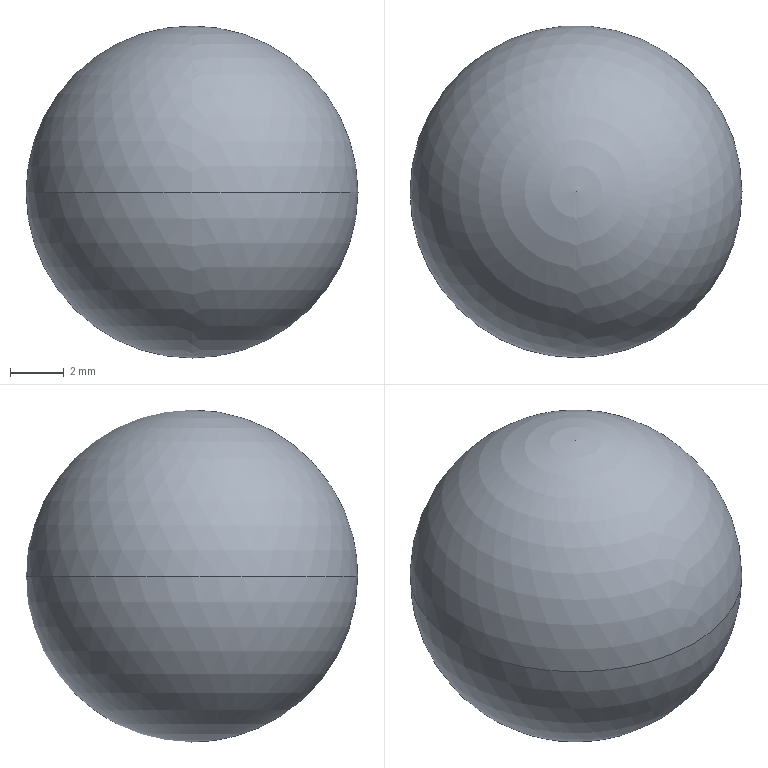Part | SolidWorks | features BaseBody 1 | 1 solid | 2 faces | box 12.303 x 12.303 x 12.303 mm | volume 975.061 mm3 | sphere 2
STEP:
#1=CARTESIAN_POINT('',(-6.152,30.,0.));
#2=VERTEX_POINT('',#1);
#3=CARTESIAN_POINT('',(6.151,30.,0.));
#4=VERTEX_POINT('',#3);
#5=CARTESIAN_POINT('',(0.,30.,0.));
#6=DIRECTION('',(0.,0.,1.));
#7=DIRECTION('',(1.,0.,0.));
#8=AXIS2_PLACEMENT_3D('',#5,#6,#7);
#9=CIRCLE('',#8,6.151);
#10=EDGE_CURVE('',#2,#4,#9,.T.);
#11=ORIENTED_EDGE('',*,*,#10,.F.);
#12=CARTESIAN_POINT('',(0.,30.,0.));
#13=DIRECTION('',(0.,0.,-1.));
#14=DIRECTION('',(0.,1.,0.));
#15=AXIS2_PLACEMENT_3D('',#12,#13,#14);
#16=CIRCLE('',#15,6.151);
#17=EDGE_CURVE('',#2,#4,#16,.T.);
#18=ORIENTED_EDGE('',*,*,#17,.T.);
#19=EDGE_LOOP('',(#11,#18));
#20=FACE_OUTER_BOUND('',#19,.T.);
#21=CARTESIAN_POINT('',(0.,30.,0.));
#22=DIRECTION('',(0.,0.,-1.));
#23=DIRECTION('',(0.,-1.,0.));
#24=AXIS2_PLACEMENT_3D('',#21,#22,#23);
#25=SPHERICAL_SURFACE('',#24,6.151);
#26=ADVANCED_FACE('',(#20),#25,.T.);
#27=ORIENTED_EDGE('',*,*,#17,.F.);
#28=ORIENTED_EDGE('',*,*,#10,.T.);
#29=EDGE_LOOP('',(#27,#28));
#30=FACE_OUTER_BOUND('',#29,.T.);
#31=CARTESIAN_POINT('',(0.,30.,0.));
#32=DIRECTION('',(0.,0.,-1.));
#33=DIRECTION('',(0.,-1.,0.));
#34=AXIS2_PLACEMENT_3D('',#31,#32,#33);
#35=SPHERICAL_SURFACE('',#34,6.151);
#36=ADVANCED_FACE('',(#30),#35,.T.);
#37=CLOSED_SHELL('',(#26,#36));
#38=MANIFOLD_SOLID_BREP('',#37);
#39=CARTESIAN_POINT('',(0.,0.,0.));
#40=DIRECTION('',(0.,0.,1.));
#41=DIRECTION('',(1.,0.,0.));
#42=AXIS2_PLACEMENT_3D('',#39,#40,#41);
#43=(LENGTH_UNIT()NAMED_UNIT(*)SI_UNIT(.MILLI.,.METRE.));
#44=UNCERTAINTY_MEASURE_WITH_UNIT(LENGTH_MEASURE(0.00001),#43,'','');
#45=(NAMED_UNIT(*)PLANE_ANGLE_UNIT()SI_UNIT($,.RADIAN.));
#46=(NAMED_UNIT(*)SI_UNIT($,.STERADIAN.)SOLID_ANGLE_UNIT());
#47=(GEOMETRIC_REPRESENTATION_CONTEXT(3)GLOBAL_UNCERTAINTY_ASSIGNED_CONTEXT((#44))GLOBAL_UNIT_ASSIGNED_CONTEXT((#43,#45,#46))REPRESENTATION_CONTEXT('',''));
#48=ADVANCED_BREP_SHAPE_REPRESENTATION('',(#38,#42),#47);